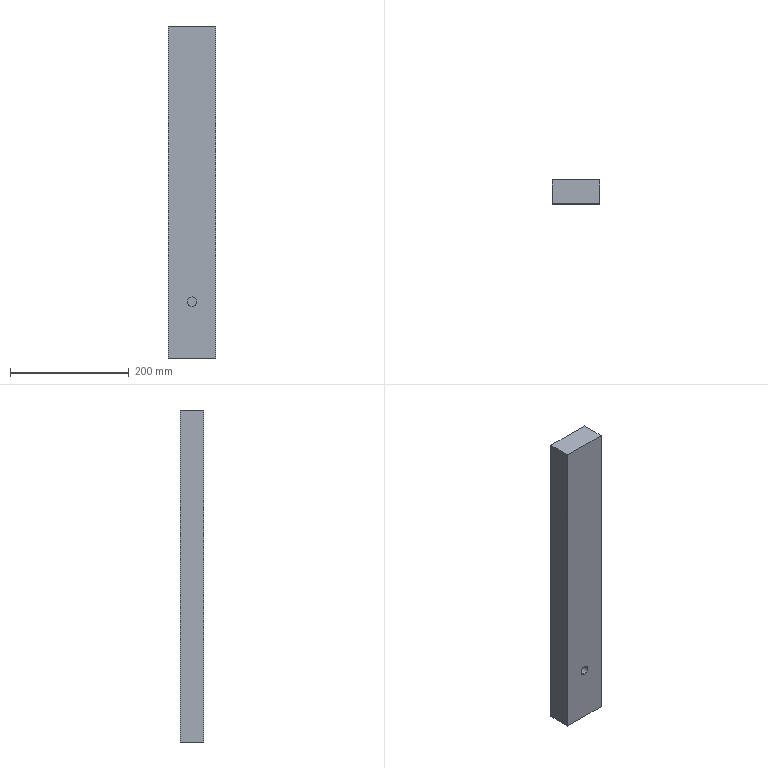Part | 1 solid | 9 faces | box 80 x 40 x 560 mm | volume 1787979 mm3 | plane 7 | cylinder 2 | commonest cylinder face diameters 16 x2
STEP:
#1=CARTESIAN_POINT('',(0.,0.,103.));
#2=VERTEX_POINT('',#1);
#3=CARTESIAN_POINT('',(0.,0.,87.));
#4=VERTEX_POINT('',#3);
#5=CARTESIAN_POINT('',(0.,0.,95.));
#6=DIRECTION('',(0.,-1.,0.));
#7=DIRECTION('',(0.,0.,-1.));
#8=AXIS2_PLACEMENT_3D('',#5,#6,#7);
#9=CIRCLE('',#8,8.);
#10=EDGE_CURVE('',#2,#4,#9,.T.);
#11=ORIENTED_EDGE('',*,*,#10,.F.);
#12=CARTESIAN_POINT('',(0.,-20.,103.));
#13=VERTEX_POINT('',#12);
#14=CARTESIAN_POINT('',(0.,0.,103.));
#15=DIRECTION('',(0.,-1.,0.));
#16=VECTOR('',#15,1000.);
#17=LINE('',#14,#16);
#18=EDGE_CURVE('',#2,#13,#17,.T.);
#19=ORIENTED_EDGE('',*,*,#18,.T.);
#20=CARTESIAN_POINT('',(0.,-20.,87.));
#21=VERTEX_POINT('',#20);
#22=CARTESIAN_POINT('',(0.,-20.,95.));
#23=DIRECTION('',(0.,-1.,0.));
#24=DIRECTION('',(0.,0.,-1.));
#25=AXIS2_PLACEMENT_3D('',#22,#23,#24);
#26=CIRCLE('',#25,8.);
#27=EDGE_CURVE('',#13,#21,#26,.T.);
#28=ORIENTED_EDGE('',*,*,#27,.T.);
#29=CARTESIAN_POINT('',(0.,0.,87.));
#30=DIRECTION('',(0.,-1.,0.));
#31=VECTOR('',#30,1000.);
#32=LINE('',#29,#31);
#33=EDGE_CURVE('',#4,#21,#32,.T.);
#34=ORIENTED_EDGE('',*,*,#33,.F.);
#35=EDGE_LOOP('',(#11,#19,#28,#34));
#36=FACE_OUTER_BOUND('',#35,.T.);
#37=CARTESIAN_POINT('',(0.,0.,95.));
#38=DIRECTION('',(0.,-1.,0.));
#39=DIRECTION('',(0.,0.,-1.));
#40=AXIS2_PLACEMENT_3D('',#37,#38,#39);
#41=CYLINDRICAL_SURFACE('',#40,8.);
#42=ADVANCED_FACE('',(#36),#41,.F.);
#43=CARTESIAN_POINT('',(40.,-20.,0.));
#44=VERTEX_POINT('',#43);
#45=CARTESIAN_POINT('',(40.,20.,0.));
#46=VERTEX_POINT('',#45);
#47=CARTESIAN_POINT('',(40.,-20.,0.));
#48=DIRECTION('',(0.,1.,0.));
#49=VECTOR('',#48,1000.);
#50=LINE('',#47,#49);
#51=EDGE_CURVE('',#44,#46,#50,.T.);
#52=ORIENTED_EDGE('',*,*,#51,.T.);
#53=CARTESIAN_POINT('',(40.,20.,560.));
#54=VERTEX_POINT('',#53);
#55=CARTESIAN_POINT('',(40.,20.,560.));
#56=DIRECTION('',(0.,0.,-1.));
#57=VECTOR('',#56,1000.);
#58=LINE('',#55,#57);
#59=EDGE_CURVE('',#54,#46,#58,.T.);
#60=ORIENTED_EDGE('',*,*,#59,.F.);
#61=CARTESIAN_POINT('',(40.,-20.,560.));
#62=VERTEX_POINT('',#61);
#63=CARTESIAN_POINT('',(40.,-20.,560.));
#64=DIRECTION('',(0.,1.,0.));
#65=VECTOR('',#64,1000.);
#66=LINE('',#63,#65);
#67=EDGE_CURVE('',#62,#54,#66,.T.);
#68=ORIENTED_EDGE('',*,*,#67,.F.);
#69=CARTESIAN_POINT('',(40.,-20.,560.));
#70=DIRECTION('',(0.,0.,-1.));
#71=VECTOR('',#70,1000.);
#72=LINE('',#69,#71);
#73=EDGE_CURVE('',#62,#44,#72,.T.);
#74=ORIENTED_EDGE('',*,*,#73,.T.);
#75=EDGE_LOOP('',(#52,#60,#68,#74));
#76=FACE_OUTER_BOUND('',#75,.T.);
#77=CARTESIAN_POINT('',(40.,-20.,560.));
#78=DIRECTION('',(-1.,0.,0.));
#79=DIRECTION('',(0.,0.,1.));
#80=AXIS2_PLACEMENT_3D('',#77,#78,#79);
#81=PLANE('',#80);
#82=ADVANCED_FACE('',(#76),#81,.F.);
#83=CARTESIAN_POINT('',(-40.,20.,0.));
#84=VERTEX_POINT('',#83);
#85=CARTESIAN_POINT('',(-40.,20.,0.));
#86=DIRECTION('',(-1.,0.,0.));
#87=VECTOR('',#86,1000.);
#88=LINE('',#85,#87);
#89=EDGE_CURVE('',#46,#84,#88,.T.);
#90=ORIENTED_EDGE('',*,*,#89,.T.);
#91=CARTESIAN_POINT('',(-40.,20.,560.));
#92=VERTEX_POINT('',#91);
#93=CARTESIAN_POINT('',(-40.,20.,560.));
#94=DIRECTION('',(0.,0.,-1.));
#95=VECTOR('',#94,1000.);
#96=LINE('',#93,#95);
#97=EDGE_CURVE('',#92,#84,#96,.T.);
#98=ORIENTED_EDGE('',*,*,#97,.F.);
#99=CARTESIAN_POINT('',(-40.,20.,560.));
#100=DIRECTION('',(-1.,0.,0.));
#101=VECTOR('',#100,1000.);
#102=LINE('',#99,#101);
#103=EDGE_CURVE('',#54,#92,#102,.T.);
#104=ORIENTED_EDGE('',*,*,#103,.F.);
#105=ORIENTED_EDGE('',*,*,#59,.T.);
#106=EDGE_LOOP('',(#90,#98,#104,#105));
#107=FACE_OUTER_BOUND('',#106,.T.);
#108=CARTESIAN_POINT('',(-40.,20.,560.));
#109=DIRECTION('',(0.,-1.,0.));
#110=DIRECTION('',(0.,0.,-1.));
#111=AXIS2_PLACEMENT_3D('',#108,#109,#110);
#112=PLANE('',#111);
#113=ADVANCED_FACE('',(#107),#112,.F.);
#114=CARTESIAN_POINT('',(-40.,-20.,0.));
#115=VERTEX_POINT('',#114);
#116=CARTESIAN_POINT('',(-40.,-20.,0.));
#117=DIRECTION('',(0.,-1.,0.));
#118=VECTOR('',#117,1000.);
#119=LINE('',#116,#118);
#120=EDGE_CURVE('',#84,#115,#119,.T.);
#121=ORIENTED_EDGE('',*,*,#120,.T.);
#122=CARTESIAN_POINT('',(-40.,-20.,560.));
#123=VERTEX_POINT('',#122);
#124=CARTESIAN_POINT('',(-40.,-20.,560.));
#125=DIRECTION('',(0.,0.,-1.));
#126=VECTOR('',#125,1000.);
#127=LINE('',#124,#126);
#128=EDGE_CURVE('',#123,#115,#127,.T.);
#129=ORIENTED_EDGE('',*,*,#128,.F.);
#130=CARTESIAN_POINT('',(-40.,-20.,560.));
#131=DIRECTION('',(0.,-1.,0.));
#132=VECTOR('',#131,1000.);
#133=LINE('',#130,#132);
#134=EDGE_CURVE('',#92,#123,#133,.T.);
#135=ORIENTED_EDGE('',*,*,#134,.F.);
#136=ORIENTED_EDGE('',*,*,#97,.T.);
#137=EDGE_LOOP('',(#121,#129,#135,#136));
#138=FACE_OUTER_BOUND('',#137,.T.);
#139=CARTESIAN_POINT('',(-40.,-20.,560.));
#140=DIRECTION('',(1.,0.,0.));
#141=DIRECTION('',(0.,0.,-1.));
#142=AXIS2_PLACEMENT_3D('',#139,#140,#141);
#143=PLANE('',#142);
#144=ADVANCED_FACE('',(#138),#143,.F.);
#145=CARTESIAN_POINT('',(0.,-20.,95.));
#146=DIRECTION('',(0.,-1.,0.));
#147=DIRECTION('',(0.,0.,-1.));
#148=AXIS2_PLACEMENT_3D('',#145,#146,#147);
#149=CIRCLE('',#148,8.);
#150=EDGE_CURVE('',#21,#13,#149,.T.);
#151=ORIENTED_EDGE('',*,*,#150,.F.);
#152=ORIENTED_EDGE('',*,*,#27,.F.);
#153=EDGE_LOOP('',(#151,#152));
#154=FACE_BOUND('',#153,.T.);
#155=CARTESIAN_POINT('',(-40.,-20.,0.));
#156=DIRECTION('',(1.,0.,0.));
#157=VECTOR('',#156,1000.);
#158=LINE('',#155,#157);
#159=EDGE_CURVE('',#115,#44,#158,.T.);
#160=ORIENTED_EDGE('',*,*,#159,.T.);
#161=ORIENTED_EDGE('',*,*,#73,.F.);
#162=CARTESIAN_POINT('',(-40.,-20.,560.));
#163=DIRECTION('',(1.,0.,0.));
#164=VECTOR('',#163,1000.);
#165=LINE('',#162,#164);
#166=EDGE_CURVE('',#123,#62,#165,.T.);
#167=ORIENTED_EDGE('',*,*,#166,.F.);
#168=ORIENTED_EDGE('',*,*,#128,.T.);
#169=EDGE_LOOP('',(#160,#161,#167,#168));
#170=FACE_OUTER_BOUND('',#169,.T.);
#171=CARTESIAN_POINT('',(-40.,-20.,560.));
#172=DIRECTION('',(0.,1.,0.));
#173=DIRECTION('',(0.,0.,1.));
#174=AXIS2_PLACEMENT_3D('',#171,#172,#173);
#175=PLANE('',#174);
#176=ADVANCED_FACE('',(#154,#170),#175,.F.);
#177=ORIENTED_EDGE('',*,*,#67,.T.);
#178=ORIENTED_EDGE('',*,*,#103,.T.);
#179=ORIENTED_EDGE('',*,*,#134,.T.);
#180=ORIENTED_EDGE('',*,*,#166,.T.);
#181=EDGE_LOOP('',(#177,#178,#179,#180));
#182=FACE_OUTER_BOUND('',#181,.T.);
#183=CARTESIAN_POINT('',(0.,0.,560.));
#184=DIRECTION('',(0.,0.,-1.));
#185=DIRECTION('',(-1.,0.,0.));
#186=AXIS2_PLACEMENT_3D('',#183,#184,#185);
#187=PLANE('',#186);
#188=ADVANCED_FACE('',(#182),#187,.F.);
#189=ORIENTED_EDGE('',*,*,#51,.F.);
#190=ORIENTED_EDGE('',*,*,#159,.F.);
#191=ORIENTED_EDGE('',*,*,#120,.F.);
#192=ORIENTED_EDGE('',*,*,#89,.F.);
#193=EDGE_LOOP('',(#189,#190,#191,#192));
#194=FACE_OUTER_BOUND('',#193,.T.);
#195=CARTESIAN_POINT('',(0.,0.,0.));
#196=DIRECTION('',(0.,0.,-1.));
#197=DIRECTION('',(-1.,0.,0.));
#198=AXIS2_PLACEMENT_3D('',#195,#196,#197);
#199=PLANE('',#198);
#200=ADVANCED_FACE('',(#194),#199,.T.);
#201=ORIENTED_EDGE('',*,*,#18,.F.);
#202=CARTESIAN_POINT('',(0.,0.,95.));
#203=DIRECTION('',(0.,-1.,0.));
#204=DIRECTION('',(0.,0.,-1.));
#205=AXIS2_PLACEMENT_3D('',#202,#203,#204);
#206=CIRCLE('',#205,8.);
#207=EDGE_CURVE('',#4,#2,#206,.T.);
#208=ORIENTED_EDGE('',*,*,#207,.F.);
#209=ORIENTED_EDGE('',*,*,#33,.T.);
#210=ORIENTED_EDGE('',*,*,#150,.T.);
#211=EDGE_LOOP('',(#201,#208,#209,#210));
#212=FACE_OUTER_BOUND('',#211,.T.);
#213=CARTESIAN_POINT('',(0.,0.,95.));
#214=DIRECTION('',(0.,-1.,0.));
#215=DIRECTION('',(0.,0.,-1.));
#216=AXIS2_PLACEMENT_3D('',#213,#214,#215);
#217=CYLINDRICAL_SURFACE('',#216,8.);
#218=ADVANCED_FACE('',(#212),#217,.F.);
#219=ORIENTED_EDGE('',*,*,#207,.T.);
#220=ORIENTED_EDGE('',*,*,#10,.T.);
#221=EDGE_LOOP('',(#219,#220));
#222=FACE_OUTER_BOUND('',#221,.T.);
#223=CARTESIAN_POINT('',(0.,0.,95.));
#224=DIRECTION('',(0.,-1.,0.));
#225=DIRECTION('',(0.,0.,-1.));
#226=AXIS2_PLACEMENT_3D('',#223,#224,#225);
#227=PLANE('',#226);
#228=ADVANCED_FACE('',(#222),#227,.T.);
#229=CLOSED_SHELL('',(#42,#82,#113,#144,#176,#188,#200,#218,#228));
#230=MANIFOLD_SOLID_BREP('',#229);
#231=CARTESIAN_POINT('',(0.,0.,0.));
#232=DIRECTION('',(0.,0.,1.));
#233=DIRECTION('',(1.,0.,0.));
#234=AXIS2_PLACEMENT_3D('',#231,#232,#233);
#235=(LENGTH_UNIT()NAMED_UNIT(*)SI_UNIT(.MILLI.,.METRE.));
#236=UNCERTAINTY_MEASURE_WITH_UNIT(LENGTH_MEASURE(0.00001),#235,'','');
#237=(NAMED_UNIT(*)PLANE_ANGLE_UNIT()SI_UNIT($,.RADIAN.));
#238=(NAMED_UNIT(*)SI_UNIT($,.STERADIAN.)SOLID_ANGLE_UNIT());
#239=(GEOMETRIC_REPRESENTATION_CONTEXT(3)GLOBAL_UNCERTAINTY_ASSIGNED_CONTEXT((#236))GLOBAL_UNIT_ASSIGNED_CONTEXT((#235,#237,#238))REPRESENTATION_CONTEXT('',''));
#240=ADVANCED_BREP_SHAPE_REPRESENTATION('',(#230,#234),#239);